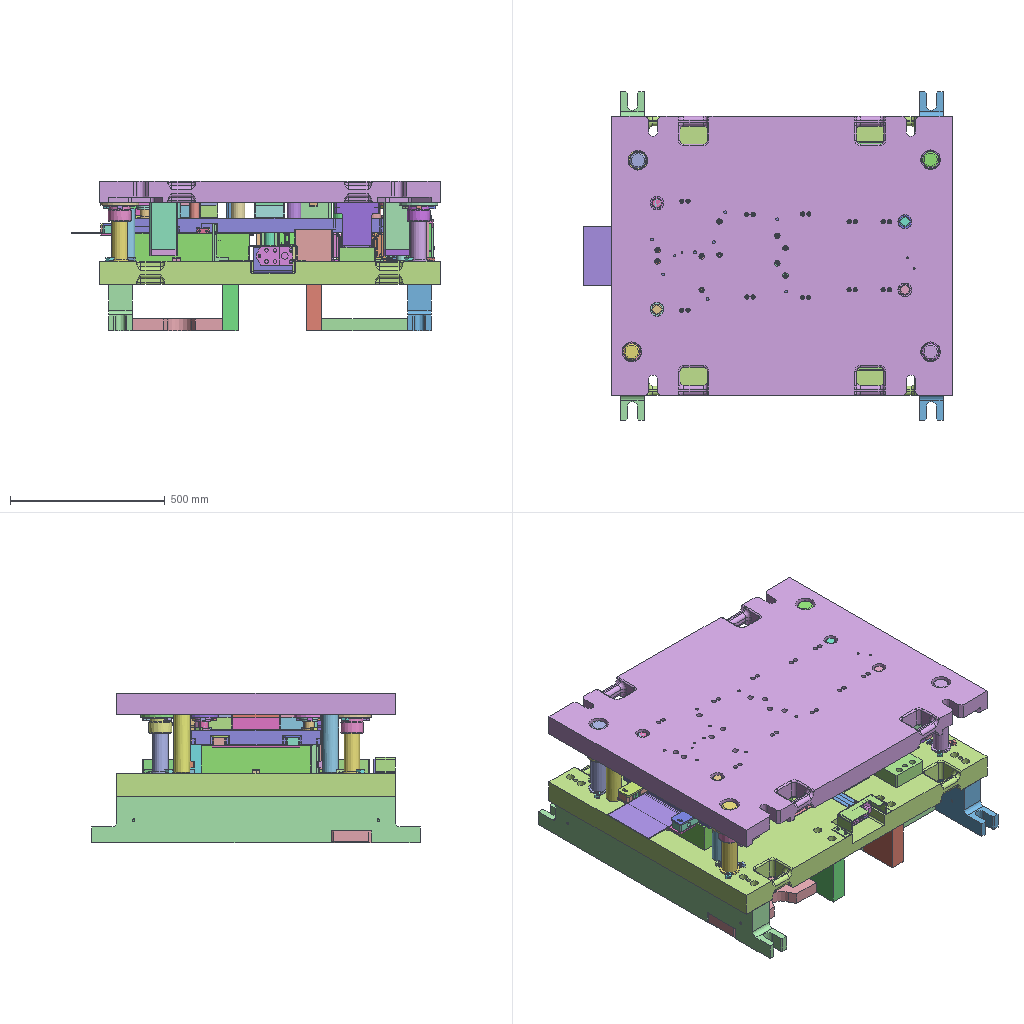Assembly | STEP file | 402 different items | 402 placed | box 1190 x 1060 x 482 mm
Parts list (item | name | quantity | parent item | size | volume):
1 | 1_id1610_x_t | x1 | in 1_x_t | 115 x 159 x 101.122 mm | 1560296 mm3
2 | 1_id1606_x_t | x1 | in 1_x_t | 114.3 x 15 x 55 mm | 89525 mm3
3 | 1_id1602_x_t | x1 | in 1_x_t | 80 x 25 x 25 mm | 40040 mm3
4 | 1_id1598_x_t | x1 | in 1_x_t | 114.3 x 15 x 55 mm | 89525 mm3
5 | 1_id1594_x_t | x1 | in 1_x_t | 15 x 15 x 10 mm | 1899 mm3
6 | 1_id1590_x_t | x1 | in 1_x_t | 61.499 x 105 x 105 mm | 262460 mm3
7 | 1_id1586_x_t | x1 | in 1_x_t | 10 x 35 x 78.24 mm | 2112 mm3
8 | 1_id1582_x_t | x1 | in 1_x_t | 120 x 140.586 x 77.52 mm | 963070 mm3
9 | 1_id1578_x_t | x1 | in 1_x_t | 100 x 20 x 45 mm | 84741 mm3
10 | 1_id1574_x_t | x1 | in 1_x_t | 10 x 10 x 28.4 mm | 1507 mm3
11 | 1_id1570_x_t | x1 | in 1_x_t | 10 x 10 x 28.4 mm | 1507 mm3
12 | 1_id1566_x_t | x1 | in 1_x_t | 10 x 10 x 28.4 mm | 1507 mm3
13 | 1_id1562_x_t | x1 | in 1_x_t | 10 x 10 x 28.4 mm | 1507 mm3
14 | 1_id1558_x_t | x1 | in 1_x_t | 30 x 16 x 16 mm | 6176 mm3
15 | 1_id1554_x_t | x1 | in 1_x_t | 115 x 20 x 66.4 mm | 145757 mm3
16 | 1_id1550_x_t | x1 | in 1_x_t | 95 x 49.497 x 48.669 mm | 78915 mm3
17 | 1_id1546_x_t | x1 | in 1_x_t | 19.05 x 114.3 x 38.1 mm | 57701 mm3
18 | 1_id1542_x_t | x1 | in 1_x_t | 115 x 159 x 101.122 mm | 1560296 mm3
19 | 1_id1538_x_t | x1 | in 1_x_t | 100 x 20 x 45 mm | 84741 mm3
20 | 1_id1534_x_t | x1 | in 1_x_t | 115 x 20 x 66.4 mm | 145757 mm3
21 | 1_id1530_x_t | x1 | in 1_x_t | 50 x 900 x 149.325 mm | 6417398 mm3
22 | 1_id1526_x_t | x1 | in 1_x_t | 63.5 x 25.4 x 25.4 mm | 33278 mm3
23 | 1_id1522_x_t | x1 | in 1_x_t | 63.5 x 25.4 x 25.4 mm | 31340 mm3
24 | 1_id1518_x_t | x1 | in 1_x_t | 303 x 50 x 6 mm | 88049 mm3
25 | 1_id1514_x_t | x1 | in 1_x_t | 31.75 x 19.4 x 24.5 mm | 13370 mm3
26 | 1_id1510_x_t | x1 | in 1_x_t | 243 x 43.296 x 24.5 mm | 189026 mm3
27 | 1_id1506_x_t | x1 | in 1_x_t | 25 x 50 x 20 mm | 19717 mm3
28 | 1_id1502_x_t | x1 | in 1_x_t | 25.4 x 25.4 x 75.5 mm | 37080 mm3
29 | 1_id1498_x_t | x1 | in 1_x_t | 25.4 x 25.4 x 75.5 mm | 37080 mm3
30 | 1_id1494_x_t | x1 | in 1_x_t | 17.227 x 16 x 69.85 mm | 12451 mm3
31 | 1_id1490_x_t | x1 | in 1_x_t | 11 x 11 x 20.4 mm | 1232 mm3
32 | 1_id1486_x_t | x1 | in 1_x_t | 156.936 x 16 x 10 mm | 21479 mm3
33 | 1_id1482_x_t | x1 | in 1_x_t | 90 x 55 x 152 mm | 644176 mm3
34 | 1_id1478_x_t | x1 | in 1_x_t | 90 x 67.5 x 20 mm | 111264 mm3
35 | 1_id1474_x_t | x1 | in 1_x_t | 32 x 32 x 52.035 mm | 37231 mm3
36 | 1_id1470_x_t | x1 | in 1_x_t | 12.7 x 12.7 x 5 mm | 467.469 mm3
37 | 1_id1466_x_t | x1 | in 1_x_t | 10.203 x 31.243 x 10 mm | 1111 mm3
38 | 1_id1462_x_t | x1 | in 1_x_t | 29.76 x 137.606 x 25 mm | 81885 mm3
39 | 1_id1458_x_t | x1 | in 1_x_t | 55 x 60 x 40 mm | 83432 mm3
40 | 1_id1454_x_t | x1 | in 1_x_t | 8 x 7.4 x 20 mm | 828.53 mm3
41 | 1_id1450_x_t | x1 | in 1_x_t | 35.397 x 13.214 x 25 mm | 9704 mm3
42 | 1_id1446_x_t | x1 | in 1_x_t | 25.4 x 38.1 x 121.275 mm | 47668 mm3
43 | 1_id1442_x_t | x1 | in 1_x_t | 10 x 35 x 78.24 mm | 2112 mm3
44 | 1_id1438_x_t | x1 | in 1_x_t | 26.187 x 24.356 x 11 mm | 2271 mm3
45 | 1_id1434_x_t | x1 | in 1_x_t | 26.187 x 24.356 x 11 mm | 2271 mm3
46 | 1_id1430_x_t | x1 | in 1_x_t | 90 x 67.5 x 20 mm | 111264 mm3
47 | 1_id1426_x_t | x1 | in 1_x_t | 90 x 55 x 152 mm | 644176 mm3
48 | 1_id1422_x_t | x1 | in 1_x_t | 90 x 67.5 x 20 mm | 111264 mm3
49 | 1_id1418_x_t | x1 | in 1_x_t | 21 x 16 x 11 mm | 2249 mm3
50 | 1_id1414_x_t | x1 | in 1_x_t | 26.187 x 24.356 x 11 mm | 2271 mm3
51 | 1_id1410_x_t | x1 | in 1_x_t | 39.688 x 39.688 x 146.05 mm | 117725 mm3
52 | 1_id1406_x_t | x1 | in 1_x_t | 26.187 x 24.356 x 11 mm | 2271 mm3
53 | 1_id1402_x_t | x1 | in 1_x_t | 90 x 55 x 152 mm | 644176 mm3
54 | 1_id1398_x_t | x1 | in 1_x_t | 90 x 67.5 x 20 mm | 111264 mm3
55 | 1_id1394_x_t | x1 | in 1_x_t | 90 x 55 x 152 mm | 644176 mm3
56 | 1_id1390_x_t | x1 | in 1_x_t | 26.187 x 24.356 x 11 mm | 2271 mm3
57 | 1_id1386_x_t | x1 | in 1_x_t | 26.187 x 24.356 x 11 mm | 2271 mm3
58 | 1_id1382_x_t | x1 | in 1_x_t | 32 x 32 x 52.035 mm | 37231 mm3
59 | 1_id1378_x_t | x1 | in 1_x_t | 32 x 32 x 52.035 mm | 37231 mm3
60 | 1_id1374_x_t | x1 | in 1_x_t | 39.688 x 39.688 x 146.05 mm | 117725 mm3
61 | 1_id1370_x_t | x1 | in 1_x_t | 26.187 x 24.356 x 11 mm | 2271 mm3
62 | 1_id1366_x_t | x1 | in 1_x_t | 26.187 x 24.356 x 11 mm | 2271 mm3
63 | 1_id1362_x_t | x1 | in 1_x_t | 80 x 25 x 25 mm | 39657 mm3
64 | 1_id1358_x_t | x1 | in 1_x_t | 50.8 x 50.8 x 190.275 mm | 342596 mm3
65 | 1_id1354_x_t | x1 | in 1_x_t | 50.8 x 50.8 x 190.275 mm | 342596 mm3
66 | 1_id1350_x_t | x1 | in 1_x_t | 50.8 x 50.8 x 190.275 mm | 342596 mm3
67 | 1_id1346_x_t | x1 | in 1_x_t | 16 x 21 x 10 mm | 2191 mm3
68 | 1_id1342_x_t | x1 | in 1_x_t | 26.187 x 24.356 x 10 mm | 2191 mm3
69 | 1_id1338_x_t | x1 | in 1_x_t | 50.8 x 50.8 x 190.275 mm | 342596 mm3
70 | 1_id1334_x_t | x1 | in 1_x_t | 20 x 30 x 25 mm | 11989 mm3
71 | 1_id1330_x_t | x1 | in 1_x_t | 209.55 x 63.5 x 50.8 mm | 52722 mm3
72 | 1_id1326_x_t | x1 | in 1_x_t | 75 x 282.347 x 6 mm | 125769 mm3
73 | 1_id1322_x_t | x1 | in 1_x_t | 31.75 x 19.4 x 24.5 mm | 13370 mm3
74 | 1_id1318_x_t | x1 | in 1_x_t | 15 x 15 x 63 mm | 7435 mm3
75 | 1_id1314_x_t | x1 | in 1_x_t | 40.468 x 31 x 10 mm | 8665 mm3
76 | 1_id1310_x_t | x1 | in 1_x_t | 50.8 x 25.4 x 120.024 mm | 43266 mm3
77 | 1_id1306_x_t | x1 | in 1_x_t | 190 x 45 x 2 mm | 16638 mm3
78 | 1_id1302_x_t | x1 | in 1_x_t | 45 x 230 x 2 mm | 20238 mm3
79 | 1_id1298_x_t | x1 | in 1_x_t | 16.123 x 43.759 x 52.166 mm | 26539 mm3
80 | 1_id1294_x_t | x1 | in 1_x_t | 6.655 x 14.782 x 12.7 mm | 658.806 mm3
81 | 1_id1290_x_t | x1 | in 1_x_t | 21.548 x 6.349 x 6.248 mm | 334.04 mm3
82 | 1_id1286_x_t | x1 | in 1_x_t | 10.535 x 11.151 x 36.727 mm | 2077 mm3
83 | 1_id1282_x_t | x1 | in 1_x_t | 41.278 x 12.093 x 11.906 mm | 2345 mm3
84 | 1_id1278_x_t | x1 | in 1_x_t | 21.548 x 6.349 x 6.248 mm | 334.04 mm3
85 | 1_id1274_x_t | x1 | in 1_x_t | 25 x 50 x 20 mm | 19717 mm3
86 | 1_id1270_x_t | x1 | in 1_x_t | 25.206 x 22.218 x 11 mm | 2271 mm3
87 | 1_id1266_x_t | x1 | in 1_x_t | 63.5 x 63.5 x 303.213 mm | 619621 mm3
88 | 1_id1262_x_t | x1 | in 1_x_t | 63.5 x 63.5 x 303.213 mm | 619621 mm3
89 | 1_id1258_x_t | x1 | in 1_x_t | 22.218 x 25.206 x 11 mm | 2271 mm3
90 | 1_id1254_x_t | x1 | in 1_x_t | 23.459 x 19.404 x 11 mm | 2271 mm3
91 | 1_id1250_x_t | x1 | in 1_x_t | 97.332 x 141.374 x 2 mm | 15084 mm3
92 | 1_id1246_x_t | x1 | in 1_x_t | 32 x 32 x 25 mm | 17096 mm3
93 | 1_id1242_x_t | x1 | in 1_x_t | 32 x 32 x 25 mm | 17096 mm3
94 | 1_id1238_x_t | x1 | in 1_x_t | 32 x 32 x 93.24 mm | 66514 mm3
95 | 1_id1234_x_t | x1 | in 1_x_t | 25 x 30 x 25 mm | 14479 mm3
96 | 1_id1230_x_t | x1 | in 1_x_t | 100 x 88.5 x 10 mm | 56263 mm3
97 | 1_id1226_x_t | x1 | in 1_x_t | 95.666 x 100 x 10 mm | 57810 mm3
98 | 1_id1222_x_t | x1 | in 1_x_t | 95.666 x 100 x 10 mm | 57810 mm3
99 | 1_id1218_x_t | x1 | in 1_x_t | 75 x 1060 x 149.325 mm | 10050016 mm3
100 | 1_id1214_x_t | x1 | in 1_x_t | 19.05 x 19.05 x 25.4 mm | 5054 mm3
101 | 1_id1210_x_t | x1 | in 1_x_t | 38 x 115.5 x 38.1 mm | 114761 mm3
102 | 1_id1206_x_t | x1 | in 1_x_t | 11 x 11 x 20.4 mm | 1232 mm3
103 | 1_id1202_x_t | x1 | in 1_x_t | 11 x 11 x 20.4 mm | 1232 mm3
104 | 1_id1198_x_t | x1 | in 1_x_t | 11 x 11 x 20.4 mm | 1232 mm3
105 | 1_id1194_x_t | x1 | in 1_x_t | 11 x 11 x 20.4 mm | 1232 mm3
106 | 1_id1190_x_t | x1 | in 1_x_t | 17.227 x 16 x 69.85 mm | 12451 mm3
107 | 1_id1186_x_t | x1 | in 1_x_t | 164.45 x 32.752 x 20.792 mm | 70018 mm3
108 | 1_id1182_x_t | x1 | in 1_x_t | 163.45 x 32.752 x 20.644 mm | 72190 mm3
109 | 1_id1178_x_t | x1 | in 1_x_t | 19 x 19 x 80 mm | 16778 mm3
110 | 1_id1174_x_t | x1 | in 1_x_t | 17.227 x 16 x 69.85 mm | 12451 mm3
111 | 1_id1170_x_t | x1 | in 1_x_t | 25.7 x 24 x 38.1 mm | 13011 mm3
112 | 1_id1166_x_t | x1 | in 1_x_t | 19 x 19 x 80 mm | 16778 mm3
113 | 1_id1162_x_t | x1 | in 1_x_t | 19 x 19 x 80 mm | 16778 mm3
114 | 1_id1158_x_t | x1 | in 1_x_t | 19 x 19 x 80 mm | 16778 mm3
115 | 1_id1154_x_t | x1 | in 1_x_t | 19 x 19 x 80 mm | 16778 mm3
116 | 1_id1150_x_t | x1 | in 1_x_t | 15.875 x 90.424 x 15.875 mm | 9884 mm3
117 | 1_id1146_x_t | x1 | in 1_x_t | 15.875 x 90.424 x 15.875 mm | 9884 mm3
118 | 1_id1142_x_t | x1 | in 1_x_t | 19 x 62.5 x 19 mm | 15480 mm3
119 | 1_id1138_x_t | x1 | in 1_x_t | 70 x 10 x 37.5 mm | 23507 mm3
120 | 1_id1134_x_t | x1 | in 1_x_t | 31.75 x 19.4 x 24.5 mm | 13370 mm3
121 | 1_id1130_x_t | x1 | in 1_x_t | 32 x 32 x 52.035 mm | 37231 mm3
122 | 1_id1126_x_t | x1 | in 1_x_t | 53.213 x 53.213 x 60.325 mm | 50805 mm3
123 | 1_id1122_x_t | x1 | in 1_x_t | 31.75 x 19.4 x 24.5 mm | 13370 mm3
124 | 1_id1118_x_t | x1 | in 1_x_t | 303 x 43.296 x 24.5 mm | 252825 mm3
125 | 1_id1114_x_t | x1 | in 1_x_t | 26.187 x 24.356 x 11 mm | 2271 mm3
126 | 1_id1110_x_t | x1 | in 1_x_t | 16 x 30 x 16 mm | 6176 mm3
127 | 1_id1106_x_t | x1 | in 1_x_t | 44.5 x 44.5 x 120 mm | 176158 mm3
128 | 1_id1102_x_t | x1 | in 1_x_t | 26.372 x 25.755 x 11 mm | 2271 mm3
129 | 1_id1098_x_t | x1 | in 1_x_t | 26.372 x 25.755 x 11 mm | 2249 mm3
130 | 1_id1094_x_t | x1 | in 1_x_t | 73.936 x 31 x 10 mm | 16212 mm3
131 | 1_id1090_x_t | x1 | in 1_x_t | 20.89 x 24.426 x 11 mm | 2271 mm3
132 | 1_id1086_x_t | x1 | in 1_x_t | 24.356 x 26.187 x 11 mm | 2249 mm3
133 | 1_id1082_x_t | x1 | in 1_x_t | 39.688 x 39.688 x 146.05 mm | 117725 mm3
134 | 1_id1078_x_t | x1 | in 1_x_t | 26.187 x 24.356 x 11 mm | 2271 mm3
135 | 1_id1074_x_t | x1 | in 1_x_t | 31.75 x 19.4 x 24.5 mm | 13473 mm3
136 | 1_id1070_x_t | x1 | in 1_x_t | 25.755 x 26.372 x 11 mm | 2271 mm3
137 | 1_id1066_x_t | x1 | in 1_x_t | 26.187 x 24.356 x 11 mm | 2271 mm3
138 | 1_id1062_x_t | x1 | in 1_x_t | 53.213 x 53.213 x 41.275 mm | 36326 mm3
139 | 1_id1058_x_t | x1 | in 1_x_t | 13.4 x 15.898 x 28.911 mm | 4184 mm3
140 | 1_id1054_x_t | x1 | in 1_x_t | 25 x 30 x 25 mm | 14479 mm3
141 | 1_id1050_x_t | x1 | in 1_x_t | 26.187 x 24.356 x 11 mm | 2271 mm3
142 | 1_id1046_x_t | x1 | in 1_x_t | 80 x 25 x 25 mm | 39657 mm3
143 | 1_id1042_x_t | x1 | in 1_x_t | 77.8 x 77.8 x 92.075 mm | 159468 mm3
144 | 1_id1038_x_t | x1 | in 1_x_t | 24.356 x 26.187 x 11 mm | 2249 mm3
145 | 1_id1034_x_t | x1 | in 1_x_t | 21 x 16 x 11 mm | 2249 mm3
146 | 1_id1030_x_t | x1 | in 1_x_t | 80 x 25 x 25 mm | 39657 mm3
147 | 1_id1026_x_t | x1 | in 1_x_t | 80 x 15 x 43 mm | 46403 mm3
148 | 1_id1022_x_t | x1 | in 1_x_t | 26.372 x 25.755 x 11 mm | 2249 mm3
149 | 1_id1018_x_t | x1 | in 1_x_t | 21 x 16 x 11 mm | 2249 mm3
150 | 1_id1014_x_t | x1 | in 1_x_t | 24.356 x 26.187 x 11 mm | 2249 mm3
151 | 1_id1010_x_t | x1 | in 1_x_t | 25.4 x 25.4 x 75.5 mm | 37080 mm3
152 | 1_id1006_x_t | x1 | in 1_x_t | 10 x 10 x 28.4 mm | 1507 mm3
153 | 1_id1002_x_t | x1 | in 1_x_t | 36.508 x 90.344 x 25 mm | 24887 mm3
154 | 1_id998_x_t | x1 | in 1_x_t | 82.5 x 86.2 x 38.01 mm | 245705 mm3
155 | 1_id994_x_t | x1 | in 1_x_t | 70 x 43.296 x 26 mm | 59877 mm3
156 | 1_id990_x_t | x1 | in 1_x_t | 21 x 16 x 11 mm | 2249 mm3
157 | 1_id986_x_t | x1 | in 1_x_t | 31.75 x 19.4 x 24.5 mm | 13370 mm3
158 | 1_id982_x_t | x1 | in 1_x_t | 15.875 x 15.875 x 5.08 mm | 809.996 mm3
159 | 1_id978_x_t | x1 | in 1_x_t | 243 x 50 x 6 mm | 70049 mm3
160 | 1_id974_x_t | x1 | in 1_x_t | 19.404 x 23.459 x 11 mm | 2271 mm3
161 | 1_id970_x_t | x1 | in 1_x_t | 25.4 x 25.4 x 75.5 mm | 37080 mm3
162 | 1_id966_x_t | x1 | in 1_x_t | 26.372 x 25.755 x 11 mm | 2271 mm3
163 | 1_id962_x_t | x1 | in 1_x_t | 50 x 25 x 20 mm | 19717 mm3
164 | 1_id958_x_t | x1 | in 1_x_t | 19 x 19 x 80 mm | 16778 mm3
165 | 1_id954_x_t | x1 | in 1_x_t | 10 x 10 x 28.4 mm | 1507 mm3
166 | 1_id950_x_t | x1 | in 1_x_t | 417 x 130 x 38.1 mm | 1861233 mm3
167 | 1_id946_x_t | x1 | in 1_x_t | 25.206 x 22.218 x 11 mm | 2271 mm3
168 | 1_id942_x_t | x1 | in 1_x_t | 19 x 19 x 80 mm | 16778 mm3
169 | 1_id938_x_t | x1 | in 1_x_t | 15.875 x 15.875 x 5.08 mm | 809.996 mm3
170 | 1_id934_x_t | x1 | in 1_x_t | 19 x 19 x 80 mm | 16778 mm3
171 | 1_id930_x_t | x1 | in 1_x_t | 26.372 x 25.755 x 11 mm | 2249 mm3
172 | 1_id926_x_t | x1 | in 1_x_t | 19 x 19 x 80 mm | 16778 mm3
173 | 1_id922_x_t | x1 | in 1_x_t | 15.876 x 15.876 x 5 mm | 818.728 mm3
174 | 1_id918_x_t | x1 | in 1_x_t | 7.4 x 8 x 20 mm | 828.53 mm3
175 | 1_id914_x_t | x1 | in 1_x_t | 15.875 x 15.875 x 5.08 mm | 809.996 mm3
176 | 1_id910_x_t | x1 | in 1_x_t | 10 x 10 x 28.4 mm | 1507 mm3
177 | 1_id906_x_t | x1 | in 1_x_t | 17 x 15 x 10 mm | 2199 mm3
178 | 1_id902_x_t | x1 | in 1_x_t | 12.423 x 12.423 x 53.975 mm | 6543 mm3
179 | 1_id898_x_t | x1 | in 1_x_t | 25.206 x 22.218 x 11 mm | 2271 mm3
180 | 1_id894_x_t | x1 | in 1_x_t | 19 x 19 x 80 mm | 16778 mm3
181 | 1_id890_x_t | x1 | in 1_x_t | 80 x 25 x 25 mm | 40040 mm3
182 | 1_id886_x_t | x1 | in 1_x_t | 15 x 15 x 10 mm | 1899 mm3
183 | 1_id882_x_t | x1 | in 1_x_t | 26.372 x 25.755 x 11 mm | 2271 mm3
184 | 1_id878_x_t | x1 | in 1_x_t | 19 x 19 x 80 mm | 16778 mm3
185 | 1_id874_x_t | x1 | in 1_x_t | 80 x 15 x 43 mm | 46403 mm3
186 | 1_id870_x_t | x1 | in 1_x_t | 4.715 x 9.009 x 51.008 mm | 844.246 mm3
187 | 1_id866_x_t | x1 | in 1_x_t | 70 x 10 x 37.5 mm | 23507 mm3
188 | 1_id862_x_t | x1 | in 1_x_t | 19.404 x 23.459 x 11 mm | 2271 mm3
189 | 1_id858_x_t | x1 | in 1_x_t | 30 x 23 x 45 mm | 21294 mm3
190 | 1_id854_x_t | x1 | in 1_x_t | 12.7 x 12.7 x 5 mm | 467.469 mm3
191 | 1_id850_x_t | x1 | in 1_x_t | 26.187 x 24.356 x 11 mm | 2271 mm3
192 | 1_id846_x_t | x1 | in 1_x_t | 17 x 15 x 10 mm | 2199 mm3
193 | 1_id842_x_t | x1 | in 1_x_t | 30 x 23 x 45 mm | 21294 mm3
194 | 1_id838_x_t | x1 | in 1_x_t | 120 x 140.586 x 77.52 mm | 963070 mm3
195 | 1_id834_x_t | x1 | in 1_x_t | 114.4 x 115 x 102.9 mm | 813776 mm3
196 | 1_id830_x_t | x1 | in 1_x_t | 26.187 x 24.356 x 11 mm | 2271 mm3
197 | 1_id826_x_t | x1 | in 1_x_t | 17.227 x 16 x 69.85 mm | 12451 mm3
198 | 1_id822_x_t | x1 | in 1_x_t | 19 x 58.09 x 19 mm | 14020 mm3
199 | 1_id818_x_t | x1 | in 1_x_t | 80 x 60 x 119 mm | 412634 mm3
200 | 1_id814_x_t | x1 | in 1_x_t | 19 x 58.09 x 19 mm | 14020 mm3
201 | 1_id810_x_t | x1 | in 1_x_t | 26.07 x 24 x 38.1 mm | 13100 mm3
202 | 1_id806_x_t | x1 | in 1_x_t | 97.332 x 141.374 x 2 mm | 15921 mm3
203 | 1_id802_x_t | x1 | in 1_x_t | 100 x 85.5 x 10 mm | 54246 mm3
204 | 1_id798_x_t | x1 | in 1_x_t | 11 x 11 x 20.4 mm | 1232 mm3
205 | 1_id794_x_t | x1 | in 1_x_t | 15.875 x 15.875 x 5.08 mm | 809.996 mm3
206 | 1_id790_x_t | x1 | in 1_x_t | 5.952 x 155.177 x 73.747 mm | 311.788 mm3
207 | 1_id786_x_t | x1 | in 1_x_t | 26.767 x 58.14 x 102.478 mm | 28325 mm3
208 | 1_id782_x_t | x1 | in 1_x_t | 11 x 11 x 20.4 mm | 1232 mm3
209 | 1_id778_x_t | x1 | in 1_x_t | 80 x 25 x 25 mm | 40040 mm3
210 | 1_id774_x_t | x1 | in 1_x_t | 26.372 x 25.755 x 11 mm | 2249 mm3
211 | 1_id770_x_t | x1 | in 1_x_t | 53.213 x 53.213 x 60.325 mm | 50805 mm3
212 | 1_id766_x_t | x1 | in 1_x_t | 15.875 x 15.875 x 5.08 mm | 809.996 mm3
213 | 1_id762_x_t | x1 | in 1_x_t | 50 x 900 x 149.325 mm | 6424966 mm3
214 | 1_id758_x_t | x1 | in 1_x_t | 63.5 x 63.5 x 303.213 mm | 619621 mm3
215 | 1_id754_x_t | x1 | in 1_x_t | 25.4 x 25.4 x 75.5 mm | 37080 mm3
216 | 1_id750_x_t | x1 | in 1_x_t | 15.875 x 15.875 x 5.08 mm | 809.996 mm3
217 | 1_id746_x_t | x1 | in 1_x_t | 10 x 10 x 28.4 mm | 1507 mm3
218 | 1_id742_x_t | x1 | in 1_x_t | 39.688 x 39.688 x 146.05 mm | 117725 mm3
219 | 1_id738_x_t | x1 | in 1_x_t | 24.356 x 26.187 x 11 mm | 2249 mm3
220 | 1_id734_x_t | x1 | in 1_x_t | 75 x 1060 x 149.325 mm | 10048750 mm3
221 | 1_id730_x_t | x1 | in 1_x_t | 32 x 32 x 93.24 mm | 66514 mm3
222 | 1_id726_x_t | x1 | in 1_x_t | 15 x 102.012 x 118 mm | 27733 mm3
223 | 1_id722_x_t | x1 | in 1_x_t | 25.4 x 25.4 x 75.5 mm | 37080 mm3
224 | 1_id718_x_t | x1 | in 1_x_t | 118 x 27.94 x 59.944 mm | 104639 mm3
225 | 1_id714_x_t | x1 | in 1_x_t | 32 x 32 x 93.24 mm | 66514 mm3
226 | 1_id710_x_t | x1 | in 1_x_t | 80 x 25 x 25 mm | 40040 mm3
227 | 1_id706_x_t | x1 | in 1_x_t | 127 x 29.369 x 82.55 mm | 82680 mm3
228 | 1_id702_x_t | x1 | in 1_x_t | 63.5 x 63.5 x 303.213 mm | 619621 mm3
229 | 1_id698_x_t | x1 | in 1_x_t | 39.688 x 39.688 x 146.05 mm | 117725 mm3
230 | 1_id694_x_t | x1 | in 1_x_t | 32 x 32 x 93.24 mm | 66514 mm3
231 | 1_id690_x_t | x1 | in 1_x_t | 32 x 92 x 31.644 mm | 71708 mm3
232 | 1_id686_x_t | x1 | in 1_x_t | 80 x 25 x 25 mm | 39657 mm3
233 | 1_id682_x_t | x1 | in 1_x_t | 56 x 128.26 x 99.32 mm | 209835 mm3
234 | 1_id678_x_t | x1 | in 1_x_t | 95 x 49.497 x 48.669 mm | 78915 mm3
235 | 1_id674_x_t | x1 | in 1_x_t | 10.203 x 31.243 x 10 mm | 1111 mm3
236 | 1_id670_x_t | x1 | in 1_x_t | 44 x 25 x 107.009 mm | 59060 mm3
237 | 1_id666_x_t | x1 | in 1_x_t | 11 x 11 x 20.4 mm | 1232 mm3
238 | 1_id662_x_t | x1 | in 1_x_t | 53.213 x 53.213 x 60.325 mm | 50805 mm3
239 | 1_id658_x_t | x1 | in 1_x_t | 69.088 x 69.85 x 41.275 mm | 100264 mm3
240 | 1_id654_x_t | x1 | in 1_x_t | 31.75 x 31.75 x 101.6 mm | 61988 mm3
241 | 1_id650_x_t | x1 | in 1_x_t | 403 x 130 x 38.1 mm | 1939605 mm3
242 | 1_id646_x_t | x1 | in 1_x_t | 49 x 79 x 5 mm | 17399 mm3
243 | 1_id642_x_t | x1 | in 1_x_t | 35 x 200 x 2 mm | 12091 mm3
244 | 1_id638_x_t | x1 | in 1_x_t | 149 x 35 x 2 mm | 8095 mm3
245 | 1_id634_x_t | x1 | in 1_x_t | 149 x 35 x 2 mm | 8095 mm3
246 | 1_id630_x_t | x1 | in 1_x_t | 44 x 25 x 107.009 mm | 59060 mm3
247 | 1_id626_x_t | x1 | in 1_x_t | 35 x 137 x 38.1 mm | 136243 mm3
248 | 1_id622_x_t | x1 | in 1_x_t | 168 x 137 x 20 mm | 442179 mm3
249 | 1_id618_x_t | x1 | in 1_x_t | 19 x 58.09 x 19 mm | 14020 mm3
250 | 1_id614_x_t | x1 | in 1_x_t | 19 x 58.09 x 19 mm | 14020 mm3
251 | 1_id610_x_t | x1 | in 1_x_t | 71 x 8 x 72 mm | 30523 mm3
252 | 1_id606_x_t | x1 | in 1_x_t | 19 x 58.09 x 19 mm | 14020 mm3
253 | 1_id602_x_t | x1 | in 1_x_t | 19 x 62.5 x 19 mm | 15480 mm3
254 | 1_id598_x_t | x1 | in 1_x_t | 35 x 137 x 38.1 mm | 136243 mm3
255 | 1_id594_x_t | x1 | in 1_x_t | 71 x 35 x 72 mm | 118326 mm3
256 | 1_id590_x_t | x1 | in 1_x_t | 15.875 x 90.424 x 15.875 mm | 9884 mm3
257 | 1_id586_x_t | x1 | in 1_x_t | 15.875 x 90.424 x 15.875 mm | 9884 mm3
258 | 1_id582_x_t | x1 | in 1_x_t | 35 x 137 x 38.1 mm | 136243 mm3
259 | 1_id578_x_t | x1 | in 1_x_t | 168 x 137 x 20 mm | 442179 mm3
260 | 1_id574_x_t | x1 | in 1_x_t | 19 x 58.09 x 19 mm | 14020 mm3
261 | 1_id570_x_t | x1 | in 1_x_t | 71 x 8 x 72 mm | 30523 mm3
262 | 1_id566_x_t | x1 | in 1_x_t | 35 x 137 x 38.1 mm | 136243 mm3
263 | 1_id562_x_t | x1 | in 1_x_t | 71 x 35 x 72 mm | 118326 mm3
264 | 1_id558_x_t | x1 | in 1_x_t | 19.05 x 114.3 x 38.1 mm | 57701 mm3
265 | 1_id554_x_t | x1 | in 1_x_t | 114.4 x 115 x 102.9 mm | 813776 mm3
266 | 1_id550_x_t | x1 | in 1_x_t | 19.05 x 114.3 x 38.1 mm | 57701 mm3
267 | 1_id546_x_t | x1 | in 1_x_t | 19.05 x 114.3 x 38.1 mm | 57701 mm3
268 | 1_id542_x_t | x1 | in 1_x_t | 11 x 11 x 20.4 mm | 1232 mm3
269 | 1_id538_x_t | x1 | in 1_x_t | 162.45 x 32.752 x 10 mm | 49655 mm3
270 | 1_id534_x_t | x1 | in 1_x_t | 163.45 x 32.752 x 10 mm | 50026 mm3
271 | 1_id530_x_t | x1 | in 1_x_t | 11 x 11 x 20.4 mm | 1232 mm3
272 | 1_id526_x_t | x1 | in 1_x_t | 11 x 11 x 20.4 mm | 1232 mm3
273 | 1_id522_x_t | x1 | in 1_x_t | 11 x 11 x 20.4 mm | 1232 mm3
274 | 1_id518_x_t | x1 | in 1_x_t | 11 x 11 x 20.4 mm | 1232 mm3
275 | 1_id514_x_t | x1 | in 1_x_t | 11 x 11 x 20.4 mm | 1232 mm3
276 | 1_id510_x_t | x1 | in 1_x_t | 11 x 11 x 20.4 mm | 1232 mm3
277 | 1_id506_x_t | x1 | in 1_x_t | 11 x 11 x 20.4 mm | 1232 mm3
278 | 1_id502_x_t | x1 | in 1_x_t | 11 x 11 x 20.4 mm | 1232 mm3
279 | 1_id498_x_t | x1 | in 1_x_t | 11 x 11 x 20.4 mm | 1232 mm3
280 | 1_id494_x_t | x1 | in 1_x_t | 11 x 11 x 20.4 mm | 1232 mm3
281 | 1_id490_x_t | x1 | in 1_x_t | 11 x 11 x 20.4 mm | 1232 mm3
282 | 1_id486_x_t | x1 | in 1_x_t | 50.8 x 50.038 x 41.275 mm | 56529 mm3
283 | 1_id482_x_t | x1 | in 1_x_t | 12.7 x 12.7 x 103.124 mm | 10701 mm3
284 | 1_id478_x_t | x1 | in 1_x_t | 125 x 105 x 10 mm | 77042 mm3
285 | 1_id474_x_t | x1 | in 1_x_t | 44.5 x 44.5 x 120 mm | 176158 mm3
286 | 1_id470_x_t | x1 | in 1_x_t | 44.5 x 44.5 x 120 mm | 176158 mm3
287 | 1_id466_x_t | x1 | in 1_x_t | 44.5 x 44.5 x 120 mm | 176158 mm3
288 | 1_id462_x_t | x1 | in 1_x_t | 44.5 x 44.5 x 120 mm | 176158 mm3
289 | 1_id458_x_t | x1 | in 1_x_t | 44.5 x 44.5 x 120 mm | 176158 mm3
290 | 1_id454_x_t | x1 | in 1_x_t | 44.5 x 44.5 x 120 mm | 176158 mm3
291 | 1_id450_x_t | x1 | in 1_x_t | 44.5 x 44.5 x 120 mm | 176158 mm3
292 | 1_id446_x_t | x1 | in 1_x_t | 44.5 x 44.5 x 120 mm | 176158 mm3
293 | 1_id442_x_t | x1 | in 1_x_t | 44.5 x 44.5 x 120 mm | 176158 mm3
294 | 1_id438_x_t | x1 | in 1_x_t | 26.187 x 24.356 x 10 mm | 2191 mm3
295 | 1_id434_x_t | x1 | in 1_x_t | 26.187 x 24.356 x 10 mm | 2191 mm3
296 | 1_id430_x_t | x1 | in 1_x_t | 125 x 105 x 10 mm | 77042 mm3
297 | 1_id426_x_t | x1 | in 1_x_t | 26.187 x 24.356 x 10 mm | 2191 mm3
298 | 1_id422_x_t | x1 | in 1_x_t | 16 x 21 x 10 mm | 2191 mm3
299 | 1_id418_x_t | x1 | in 1_x_t | 77.8 x 77.8 x 92.075 mm | 159468 mm3
300 | 1_id414_x_t | x1 | in 1_x_t | 77.8 x 77.8 x 92.075 mm | 159468 mm3
301 | 1_id410_x_t | x1 | in 1_x_t | 125 x 105 x 10 mm | 77042 mm3
302 | 1_id406_x_t | x1 | in 1_x_t | 16 x 21 x 10 mm | 2191 mm3
303 | 1_id402_x_t | x1 | in 1_x_t | 26.187 x 24.356 x 10 mm | 2191 mm3
304 | 1_id398_x_t | x1 | in 1_x_t | 26.187 x 24.356 x 10 mm | 2191 mm3
305 | 1_id394_x_t | x1 | in 1_x_t | 77.8 x 77.8 x 92.075 mm | 159468 mm3
306 | 1_id390_x_t | x1 | in 1_x_t | 26.187 x 24.356 x 10 mm | 2191 mm3
307 | 1_id386_x_t | x1 | in 1_x_t | 125 x 105 x 10 mm | 77042 mm3
308 | 1_id382_x_t | x1 | in 1_x_t | 16 x 21 x 10 mm | 2191 mm3
309 | 1_id378_x_t | x1 | in 1_x_t | 26.187 x 24.356 x 10 mm | 2191 mm3
310 | 1_id374_x_t | x1 | in 1_x_t | 68.793 x 69.35 x 5 mm | 16032 mm3
311 | 1_id370_x_t | x1 | in 1_x_t | 9.15 x 21.764 x 3.075 mm | 435.444 mm3
312 | 1_id366_x_t | x1 | in 1_x_t | 48.382 x 188.49 x 8.554 mm | 28332 mm3
313 | 1_id362_x_t | x1 | in 1_x_t | 8.17 x 3.075 x 8.17 mm | 161.205 mm3
314 | PARTBODY_id358_x_t | x1 | in 1_x_t | 48 x 47.1 x 81.415 mm | 28561 mm3
315 | PARTBODY_id354_x_t | x1 | in 1_x_t | 48 x 47.1 x 81.415 mm | 28561 mm3
316 | 1_id350_x_t | x1 | in 1_x_t | 8.17 x 3.075 x 8.17 mm | 161.205 mm3
317 | 1_id346_x_t | x1 | in 1_x_t | 48.382 x 188.49 x 8.554 mm | 28333 mm3
318 | 1_id342_x_t | x1 | in 1_x_t | 8.17 x 3.075 x 8.17 mm | 161.205 mm3
319 | 1_id338_x_t | x1 | in 1_x_t | 9.576 x 9.576 x 3.075 mm | 221.455 mm3
320 | PARTBODY_id334_x_t | x1 | in 1_x_t | 48 x 47.1 x 81.415 mm | 28561 mm3
321 | PARTBODY_id330_x_t | x1 | in 1_x_t | 48 x 46.9 x 81.415 mm | 29174 mm3
322 | 1_id326_x_t | x1 | in 1_x_t | 9.576 x 9.576 x 3.075 mm | 221.455 mm3
323 | 1_id322_x_t | x1 | in 1_x_t | 8.17 x 3.075 x 8.17 mm | 161.205 mm3
324 | 1_id318_x_t | x1 | in 1_x_t | 8.17 x 3.075 x 8.17 mm | 161.205 mm3
325 | PARTBODY_id314_x_t | x1 | in 1_x_t | 48 x 48.7 x 81.415 mm | 29466 mm3
326 | PARTBODY_id310_x_t | x1 | in 1_x_t | 48 x 47.1 x 81.415 mm | 29206 mm3
327 | 1_id306_x_t | x1 | in 1_x_t | 8.17 x 3.075 x 8.17 mm | 161.205 mm3
328 | 1_id302_x_t | x1 | in 1_x_t | 8.17 x 3.075 x 8.17 mm | 161.205 mm3
329 | 1_id298_x_t | x1 | in 1_x_t | 499.877 x 188.495 x 8.554 mm | 279674 mm3
330 | PARTBODY_id294_x_t | x1 | in 1_x_t | 48 x 47.1 x 81.415 mm | 29206 mm3
331 | 1_id290_x_t | x1 | in 1_x_t | 4.043 x 0.7546 x 0.00007192 mm | 0.000006524 mm3
332 | 1_id286_x_t | x1 | in 1_x_t | 8.95 x 3 x 8.95 mm | 188.737 mm3
333 | 1_id282_x_t | x1 | in 1_x_t | 143.3 x 84 x 105 mm | 430781 mm3
334 | 1_id278_x_t | x1 | in 1_x_t | 13 x 14 x 43 mm | 5330 mm3
335 | 1_id274_x_t | x1 | in 1_x_t | 13 x 14 x 43 mm | 5330 mm3
336 | 1_id270_x_t | x1 | in 1_x_t | 20 x 20 x 20 mm | 5374 mm3
337 | 1_id266_x_t | x1 | in 1_x_t | 70.8 x 244.8 x 3 mm | 48416 mm3
338 | 1_id262_x_t | x1 | in 1_x_t | 11 x 11 x 48.205 mm | 3006 mm3
339 | 1_id258_x_t | x1 | in 1_x_t | 11 x 11 x 4 mm | 380.137 mm3
340 | 1_id254_x_t | x1 | in 1_x_t | 11 x 11 x 48.205 mm | 3006 mm3
341 | 1_id250_x_t | x1 | in 1_x_t | 11 x 11 x 48.205 mm | 3006 mm3
342 | 1_id246_x_t | x1 | in 1_x_t | 11 x 11 x 48.205 mm | 3006 mm3
343 | 1_id242_x_t | x1 | in 1_x_t | 11 x 11 x 48.205 mm | 3006 mm3
344 | 1_id238_x_t | x1 | in 1_x_t | 11 x 11 x 48.205 mm | 3006 mm3
345 | 1_id234_x_t | x1 | in 1_x_t | 11 x 11 x 48.205 mm | 3006 mm3
346 | 1_id230_x_t | x1 | in 1_x_t | 11 x 11 x 48.205 mm | 3006 mm3
347 | 1_id226_x_t | x1 | in 1_x_t | 11 x 11 x 48.205 mm | 3006 mm3
348 | 1_id222_x_t | x1 | in 1_x_t | 11 x 11 x 48.205 mm | 3006 mm3
349 | 1_id218_x_t | x1 | in 1_x_t | 11 x 11 x 48.205 mm | 3006 mm3
350 | 1_id214_x_t | x1 | in 1_x_t | 11 x 11 x 48.205 mm | 3006 mm3
351 | 1_id210_x_t | x1 | in 1_x_t | 48 x 173.045 x 42.999 mm | 28963 mm3
352 | 1_id206_x_t | x1 | in 1_x_t | 68 x 186 x 10 mm | 120598 mm3
353 | 1_id202_x_t | x1 | in 1_x_t | 68 x 186 x 38.1 mm | 377160 mm3
354 | 1_id198_x_t | x1 | in 1_x_t | 51.017 x 50.028 x 5 mm | 8124 mm3
355 | 1_id194_x_t | x1 | in 1_x_t | 1100 x 900 x 68 mm | 61756631 mm3
356 | 1_id190_x_t | x1 | in 1_x_t | 98 x 265 x 10 mm | 250017 mm3
357 | 1_id186_x_t | x1 | in 1_x_t | 68 x 155 x 10 mm | 99518 mm3
358 | 1_id182_x_t | x1 | in 1_x_t | 68 x 185 x 10 mm | 112684 mm3
359 | 1_id178_x_t | x1 | in 1_x_t | 68 x 185 x 38.1 mm | 347953 mm3
360 | 1_id174_x_t | x1 | in 1_x_t | 68 x 155 x 38.1 mm | 290380 mm3
361 | 1_id170_x_t | x1 | in 1_x_t | 98 x 265 x 38.1 mm | 540767 mm3
362 | 1_id166_x_t | x1 | in 1_x_t | 145 x 95 x 182.773 mm | 1439851 mm3
363 | 1_id162_x_t | x1 | in 1_x_t | 145 x 95 x 182.773 mm | 1440904 mm3
364 | 1_id158_x_t | x1 | in 1_x_t | 114.3 x 103.32 x 163.553 mm | 1068364 mm3
365 | 1_id154_x_t | x1 | in 1_x_t | 114.3 x 103.32 x 163.553 mm | 1067173 mm3
366 | 1_id150_x_t | x1 | in 1_x_t | 51 x 202 x 97.035 mm | 913093 mm3
367 | 1_id146_x_t | x1 | in 1_x_t | 35 x 131.5 x 97.111 mm | 189227 mm3
368 | 1_id142_x_t | x1 | in 1_x_t | 35 x 130.5 x 97.111 mm | 188320 mm3
369 | 1_id138_x_t | x1 | in 1_x_t | 36 x 66 x 86.679 mm | 191132 mm3
370 | 1_id134_x_t | x1 | in 1_x_t | 35.8 x 65.8 x 6 mm | 12762 mm3
371 | 1_id130_x_t | x1 | in 1_x_t | 925 x 416 x 45.006 mm | 11838970 mm3
372 | 1_id126_x_t | x1 | in 1_x_t | 400 x 355 x 90 mm | 10202987 mm3
373 | 1_id122_x_t | x1 | in 1_x_t | 35 x 115.5 x 38.1 mm | 107010 mm3
374 | 1_id118_x_t | x1 | in 1_x_t | 96 x 38 x 70.5 mm | 174436 mm3
375 | 1_id114_x_t | x1 | in 1_x_t | 71 x 245 x 22.4 mm | 320775 mm3
376 | 1_id110_x_t | x1 | in 1_x_t | 35 x 115.5 x 38.1 mm | 106763 mm3
377 | 1_id106_x_t | x1 | in 1_x_t | 38 x 115.5 x 38.1 mm | 113928 mm3
378 | 1_id102_x_t | x1 | in 1_x_t | 50 x 80 x 38.1 mm | 121881 mm3
379 | 1_id98_x_t | x1 | in 1_x_t | 96 x 38 x 70.5 mm | 174436 mm3
380 | 1_id94_x_t | x1 | in 1_x_t | 1100 x 900 x 75 mm | 64161476 mm3
381 | 1_id90_x_t | x1 | in 1_x_t | 48 x 173.045 x 42.934 mm | 28634 mm3
382 | 1_id86_x_t | x1 | in 1_x_t | 48 x 173.045 x 42.999 mm | 28624 mm3
383 | 1_id82_x_t | x1 | in 1_x_t | 80 x 230 x 101 mm | 1363447 mm3
384 | 1_id78_x_t | x1 | in 1_x_t | 80 x 230 x 4 mm | 72058 mm3
385 | 1_id74_x_t | x1 | in 1_x_t | 56 x 195 x 126 mm | 1101348 mm3
386 | 1_id70_x_t | x1 | in 1_x_t | 56 x 195 x 4.5 mm | 48168 mm3
387 | 1_id66_x_t | x1 | in 1_x_t | 48 x 173.045 x 42.999 mm | 28624 mm3
388 | 1_id62_x_t | x1 | in 1_x_t | 72 x 85 x 105 mm | 283891 mm3
389 | 1_id58_x_t | x1 | in 1_x_t | 66 x 85 x 105 mm | 245163 mm3
390 | 1_id54_x_t | x1 | in 1_x_t | 57.15 x 38 x 85.5 mm | 141794 mm3
391 | 1_id50_x_t | x1 | in 1_x_t | 57.15 x 38 x 85.5 mm | 143205 mm3
392 | 1_id46_x_t | x1 | in 1_x_t | 57.15 x 38 x 85.5 mm | 141792 mm3
393 | 1_id42_x_t | x1 | in 1_x_t | 57.15 x 38 x 85.5 mm | 143246 mm3
394 | 1_id38_x_t | x1 | in 1_x_t | 9.15 x 21.764 x 3.075 mm | 435.444 mm3
395 | 1_id34_x_t | x1 | in 1_x_t | 9.15 x 21.764 x 3.075 mm | 435.444 mm3
396 | 1_id30_x_t | x1 | in 1_x_t | 9.15 x 21.764 x 3.075 mm | 435.444 mm3
397 | 1_id26_x_t | x1 | in 1_x_t | 9.15 x 21.764 x 3.075 mm | 435.444 mm3
398 | 1_id22_x_t | x1 | in 1_x_t | 9.15 x 21.764 x 3.075 mm | 435.444 mm3
399 | 1_id18_x_t | x1 | in 1_x_t | 9.15 x 21.764 x 3.075 mm | 435.444 mm3
400 | 1_id14_x_t | x1 | in 1_x_t | 9.15 x 21.764 x 3.075 mm | 435.444 mm3
401 | 1_id10_x_t | x1 | in 1_x_t | 9.15 x 21.764 x 3.075 mm | 435.444 mm3
402 | 1_id6_x_t | x1 | in 1_x_t | 9.15 x 21.764 x 3.075 mm | 435.444 mm3
Placements (level | parent | child | x y z in mm | rotation matrix by rows), first 180 of 402 lines:
1 | 1_x_t | 1_id1610_x_t | 0.0 0.0 0.0 | 1 0 0 0 1 0 0 0 1
1 | 1_x_t | 1_id1606_x_t | 0.0 0.0 0.0 | 1 0 0 0 1 0 0 0 1
1 | 1_x_t | 1_id1602_x_t | 0.0 0.0 0.0 | 1 0 0 0 1 0 0 0 1
1 | 1_x_t | 1_id1598_x_t | 0.0 0.0 0.0 | 1 0 0 0 1 0 0 0 1
1 | 1_x_t | 1_id1594_x_t | 0.0 0.0 0.0 | 1 0 0 0 1 0 0 0 1
1 | 1_x_t | 1_id1590_x_t | 0.0 0.0 0.0 | 1 0 0 0 1 0 0 0 1
1 | 1_x_t | 1_id1586_x_t | 0.0 0.0 0.0 | 1 0 0 0 1 0 0 0 1
1 | 1_x_t | 1_id1582_x_t | 0.0 0.0 0.0 | 1 0 0 0 1 0 0 0 1
1 | 1_x_t | 1_id1578_x_t | 0.0 0.0 0.0 | 1 0 0 0 1 0 0 0 1
1 | 1_x_t | 1_id1574_x_t | 0.0 0.0 0.0 | 1 0 0 0 1 0 0 0 1
1 | 1_x_t | 1_id1570_x_t | 0.0 0.0 0.0 | 1 0 0 0 1 0 0 0 1
1 | 1_x_t | 1_id1566_x_t | 0.0 0.0 0.0 | 1 0 0 0 1 0 0 0 1
1 | 1_x_t | 1_id1562_x_t | 0.0 0.0 0.0 | 1 0 0 0 1 0 0 0 1
1 | 1_x_t | 1_id1558_x_t | 0.0 0.0 0.0 | 1 0 0 0 1 0 0 0 1
1 | 1_x_t | 1_id1554_x_t | 0.0 0.0 0.0 | 1 0 0 0 1 0 0 0 1
1 | 1_x_t | 1_id1550_x_t | 0.0 0.0 0.0 | 1 0 0 0 1 0 0 0 1
1 | 1_x_t | 1_id1546_x_t | 0.0 0.0 0.0 | 1 0 0 0 1 0 0 0 1
1 | 1_x_t | 1_id1542_x_t | 0.0 0.0 0.0 | 1 0 0 0 1 0 0 0 1
1 | 1_x_t | 1_id1538_x_t | 0.0 0.0 0.0 | 1 0 0 0 1 0 0 0 1
1 | 1_x_t | 1_id1534_x_t | 0.0 0.0 0.0 | 1 0 0 0 1 0 0 0 1
1 | 1_x_t | 1_id1530_x_t | 0.0 0.0 0.0 | 1 0 0 0 1 0 0 0 1
1 | 1_x_t | 1_id1526_x_t | 0.0 0.0 0.0 | 1 0 0 0 1 0 0 0 1
1 | 1_x_t | 1_id1522_x_t | 0.0 0.0 0.0 | 1 0 0 0 1 0 0 0 1
1 | 1_x_t | 1_id1518_x_t | 0.0 0.0 0.0 | 1 0 0 0 1 0 0 0 1
1 | 1_x_t | 1_id1514_x_t | 0.0 0.0 0.0 | 1 0 0 0 1 0 0 0 1
1 | 1_x_t | 1_id1510_x_t | 0.0 0.0 0.0 | 1 0 0 0 1 0 0 0 1
1 | 1_x_t | 1_id1506_x_t | 0.0 0.0 0.0 | 1 0 0 0 1 0 0 0 1
1 | 1_x_t | 1_id1502_x_t | 0.0 0.0 0.0 | 1 0 0 0 1 0 0 0 1
1 | 1_x_t | 1_id1498_x_t | 0.0 0.0 0.0 | 1 0 0 0 1 0 0 0 1
1 | 1_x_t | 1_id1494_x_t | 0.0 0.0 0.0 | 1 0 0 0 1 0 0 0 1
1 | 1_x_t | 1_id1490_x_t | 0.0 0.0 0.0 | 1 0 0 0 1 0 0 0 1
1 | 1_x_t | 1_id1486_x_t | 0.0 0.0 0.0 | 1 0 0 0 1 0 0 0 1
1 | 1_x_t | 1_id1482_x_t | 0.0 0.0 0.0 | 1 0 0 0 1 0 0 0 1
1 | 1_x_t | 1_id1478_x_t | 0.0 0.0 0.0 | 1 0 0 0 1 0 0 0 1
1 | 1_x_t | 1_id1474_x_t | 0.0 0.0 0.0 | 1 0 0 0 1 0 0 0 1
1 | 1_x_t | 1_id1470_x_t | 0.0 0.0 0.0 | 1 0 0 0 1 0 0 0 1
1 | 1_x_t | 1_id1466_x_t | 0.0 0.0 0.0 | 1 0 0 0 1 0 0 0 1
1 | 1_x_t | 1_id1462_x_t | 0.0 0.0 0.0 | 1 0 0 0 1 0 0 0 1
1 | 1_x_t | 1_id1458_x_t | 0.0 0.0 0.0 | 1 0 0 0 1 0 0 0 1
1 | 1_x_t | 1_id1454_x_t | 0.0 0.0 0.0 | 1 0 0 0 1 0 0 0 1
1 | 1_x_t | 1_id1450_x_t | 0.0 0.0 0.0 | 1 0 0 0 1 0 0 0 1
1 | 1_x_t | 1_id1446_x_t | 0.0 0.0 0.0 | 1 0 0 0 1 0 0 0 1
1 | 1_x_t | 1_id1442_x_t | 0.0 0.0 0.0 | 1 0 0 0 1 0 0 0 1
1 | 1_x_t | 1_id1438_x_t | 0.0 0.0 0.0 | 1 0 0 0 1 0 0 0 1
1 | 1_x_t | 1_id1434_x_t | 0.0 0.0 0.0 | 1 0 0 0 1 0 0 0 1
1 | 1_x_t | 1_id1430_x_t | 0.0 0.0 0.0 | 1 0 0 0 1 0 0 0 1
1 | 1_x_t | 1_id1426_x_t | 0.0 0.0 0.0 | 1 0 0 0 1 0 0 0 1
1 | 1_x_t | 1_id1422_x_t | 0.0 0.0 0.0 | 1 0 0 0 1 0 0 0 1
1 | 1_x_t | 1_id1418_x_t | 0.0 0.0 0.0 | 1 0 0 0 1 0 0 0 1
1 | 1_x_t | 1_id1414_x_t | 0.0 0.0 0.0 | 1 0 0 0 1 0 0 0 1
1 | 1_x_t | 1_id1410_x_t | 0.0 0.0 0.0 | 1 0 0 0 1 0 0 0 1
1 | 1_x_t | 1_id1406_x_t | 0.0 0.0 0.0 | 1 0 0 0 1 0 0 0 1
1 | 1_x_t | 1_id1402_x_t | 0.0 0.0 0.0 | 1 0 0 0 1 0 0 0 1
1 | 1_x_t | 1_id1398_x_t | 0.0 0.0 0.0 | 1 0 0 0 1 0 0 0 1
1 | 1_x_t | 1_id1394_x_t | 0.0 0.0 0.0 | 1 0 0 0 1 0 0 0 1
1 | 1_x_t | 1_id1390_x_t | 0.0 0.0 0.0 | 1 0 0 0 1 0 0 0 1
1 | 1_x_t | 1_id1386_x_t | 0.0 0.0 0.0 | 1 0 0 0 1 0 0 0 1
1 | 1_x_t | 1_id1382_x_t | 0.0 0.0 0.0 | 1 0 0 0 1 0 0 0 1
1 | 1_x_t | 1_id1378_x_t | 0.0 0.0 0.0 | 1 0 0 0 1 0 0 0 1
1 | 1_x_t | 1_id1374_x_t | 0.0 0.0 0.0 | 1 0 0 0 1 0 0 0 1
1 | 1_x_t | 1_id1370_x_t | 0.0 0.0 0.0 | 1 0 0 0 1 0 0 0 1
1 | 1_x_t | 1_id1366_x_t | 0.0 0.0 0.0 | 1 0 0 0 1 0 0 0 1
1 | 1_x_t | 1_id1362_x_t | 0.0 0.0 0.0 | 1 0 0 0 1 0 0 0 1
1 | 1_x_t | 1_id1358_x_t | 0.0 0.0 0.0 | 1 0 0 0 1 0 0 0 1
1 | 1_x_t | 1_id1354_x_t | 0.0 0.0 0.0 | 1 0 0 0 1 0 0 0 1
1 | 1_x_t | 1_id1350_x_t | 0.0 0.0 0.0 | 1 0 0 0 1 0 0 0 1
1 | 1_x_t | 1_id1346_x_t | 0.0 0.0 0.0 | 1 0 0 0 1 0 0 0 1
1 | 1_x_t | 1_id1342_x_t | 0.0 0.0 0.0 | 1 0 0 0 1 0 0 0 1
1 | 1_x_t | 1_id1338_x_t | 0.0 0.0 0.0 | 1 0 0 0 1 0 0 0 1
1 | 1_x_t | 1_id1334_x_t | 0.0 0.0 0.0 | 1 0 0 0 1 0 0 0 1
1 | 1_x_t | 1_id1330_x_t | 0.0 0.0 0.0 | 1 0 0 0 1 0 0 0 1
1 | 1_x_t | 1_id1326_x_t | 0.0 0.0 0.0 | 1 0 0 0 1 0 0 0 1
1 | 1_x_t | 1_id1322_x_t | 0.0 0.0 0.0 | 1 0 0 0 1 0 0 0 1
1 | 1_x_t | 1_id1318_x_t | 0.0 0.0 0.0 | 1 0 0 0 1 0 0 0 1
1 | 1_x_t | 1_id1314_x_t | 0.0 0.0 0.0 | 1 0 0 0 1 0 0 0 1
1 | 1_x_t | 1_id1310_x_t | 0.0 0.0 0.0 | 1 0 0 0 1 0 0 0 1
1 | 1_x_t | 1_id1306_x_t | 0.0 0.0 0.0 | 1 0 0 0 1 0 0 0 1
1 | 1_x_t | 1_id1302_x_t | 0.0 0.0 0.0 | 1 0 0 0 1 0 0 0 1
1 | 1_x_t | 1_id1298_x_t | 0.0 0.0 0.0 | 1 0 0 0 1 0 0 0 1
1 | 1_x_t | 1_id1294_x_t | 0.0 0.0 0.0 | 1 0 0 0 1 0 0 0 1
1 | 1_x_t | 1_id1290_x_t | 0.0 0.0 0.0 | 1 0 0 0 1 0 0 0 1
1 | 1_x_t | 1_id1286_x_t | 0.0 0.0 0.0 | 1 0 0 0 1 0 0 0 1
1 | 1_x_t | 1_id1282_x_t | 0.0 0.0 0.0 | 1 0 0 0 1 0 0 0 1
1 | 1_x_t | 1_id1278_x_t | 0.0 0.0 0.0 | 1 0 0 0 1 0 0 0 1
1 | 1_x_t | 1_id1274_x_t | 0.0 0.0 0.0 | 1 0 0 0 1 0 0 0 1
1 | 1_x_t | 1_id1270_x_t | 0.0 0.0 0.0 | 1 0 0 0 1 0 0 0 1
1 | 1_x_t | 1_id1266_x_t | 0.0 0.0 0.0 | 1 0 0 0 1 0 0 0 1
1 | 1_x_t | 1_id1262_x_t | 0.0 0.0 0.0 | 1 0 0 0 1 0 0 0 1
1 | 1_x_t | 1_id1258_x_t | 0.0 0.0 0.0 | 1 0 0 0 1 0 0 0 1
1 | 1_x_t | 1_id1254_x_t | 0.0 0.0 0.0 | 1 0 0 0 1 0 0 0 1
1 | 1_x_t | 1_id1250_x_t | 0.0 0.0 0.0 | 1 0 0 0 1 0 0 0 1
1 | 1_x_t | 1_id1246_x_t | 0.0 0.0 0.0 | 1 0 0 0 1 0 0 0 1
1 | 1_x_t | 1_id1242_x_t | 0.0 0.0 0.0 | 1 0 0 0 1 0 0 0 1
1 | 1_x_t | 1_id1238_x_t | 0.0 0.0 0.0 | 1 0 0 0 1 0 0 0 1
1 | 1_x_t | 1_id1234_x_t | 0.0 0.0 0.0 | 1 0 0 0 1 0 0 0 1
1 | 1_x_t | 1_id1230_x_t | 0.0 0.0 0.0 | 1 0 0 0 1 0 0 0 1
1 | 1_x_t | 1_id1226_x_t | 0.0 0.0 0.0 | 1 0 0 0 1 0 0 0 1
1 | 1_x_t | 1_id1222_x_t | 0.0 0.0 0.0 | 1 0 0 0 1 0 0 0 1
1 | 1_x_t | 1_id1218_x_t | 0.0 0.0 0.0 | 1 0 0 0 1 0 0 0 1
1 | 1_x_t | 1_id1214_x_t | 0.0 0.0 0.0 | 1 0 0 0 1 0 0 0 1
1 | 1_x_t | 1_id1210_x_t | 0.0 0.0 0.0 | 1 0 0 0 1 0 0 0 1
1 | 1_x_t | 1_id1206_x_t | 0.0 0.0 0.0 | 1 0 0 0 1 0 0 0 1
1 | 1_x_t | 1_id1202_x_t | 0.0 0.0 0.0 | 1 0 0 0 1 0 0 0 1
1 | 1_x_t | 1_id1198_x_t | 0.0 0.0 0.0 | 1 0 0 0 1 0 0 0 1
1 | 1_x_t | 1_id1194_x_t | 0.0 0.0 0.0 | 1 0 0 0 1 0 0 0 1
1 | 1_x_t | 1_id1190_x_t | 0.0 0.0 0.0 | 1 0 0 0 1 0 0 0 1
1 | 1_x_t | 1_id1186_x_t | 0.0 0.0 0.0 | 1 0 0 0 1 0 0 0 1
1 | 1_x_t | 1_id1182_x_t | 0.0 0.0 0.0 | 1 0 0 0 1 0 0 0 1
1 | 1_x_t | 1_id1178_x_t | 0.0 0.0 0.0 | 1 0 0 0 1 0 0 0 1
1 | 1_x_t | 1_id1174_x_t | 0.0 0.0 0.0 | 1 0 0 0 1 0 0 0 1
1 | 1_x_t | 1_id1170_x_t | 0.0 0.0 0.0 | 1 0 0 0 1 0 0 0 1
1 | 1_x_t | 1_id1166_x_t | 0.0 0.0 0.0 | 1 0 0 0 1 0 0 0 1
1 | 1_x_t | 1_id1162_x_t | 0.0 0.0 0.0 | 1 0 0 0 1 0 0 0 1
1 | 1_x_t | 1_id1158_x_t | 0.0 0.0 0.0 | 1 0 0 0 1 0 0 0 1
1 | 1_x_t | 1_id1154_x_t | 0.0 0.0 0.0 | 1 0 0 0 1 0 0 0 1
1 | 1_x_t | 1_id1150_x_t | 0.0 0.0 0.0 | 1 0 0 0 1 0 0 0 1
1 | 1_x_t | 1_id1146_x_t | 0.0 0.0 0.0 | 1 0 0 0 1 0 0 0 1
1 | 1_x_t | 1_id1142_x_t | 0.0 0.0 0.0 | 1 0 0 0 1 0 0 0 1
1 | 1_x_t | 1_id1138_x_t | 0.0 0.0 0.0 | 1 0 0 0 1 0 0 0 1
1 | 1_x_t | 1_id1134_x_t | 0.0 0.0 0.0 | 1 0 0 0 1 0 0 0 1
1 | 1_x_t | 1_id1130_x_t | 0.0 0.0 0.0 | 1 0 0 0 1 0 0 0 1
1 | 1_x_t | 1_id1126_x_t | 0.0 0.0 0.0 | 1 0 0 0 1 0 0 0 1
1 | 1_x_t | 1_id1122_x_t | 0.0 0.0 0.0 | 1 0 0 0 1 0 0 0 1
1 | 1_x_t | 1_id1118_x_t | 0.0 0.0 0.0 | 1 0 0 0 1 0 0 0 1
1 | 1_x_t | 1_id1114_x_t | 0.0 0.0 0.0 | 1 0 0 0 1 0 0 0 1
1 | 1_x_t | 1_id1110_x_t | 0.0 0.0 0.0 | 1 0 0 0 1 0 0 0 1
1 | 1_x_t | 1_id1106_x_t | 0.0 0.0 0.0 | 1 0 0 0 1 0 0 0 1
1 | 1_x_t | 1_id1102_x_t | 0.0 0.0 0.0 | 1 0 0 0 1 0 0 0 1
1 | 1_x_t | 1_id1098_x_t | 0.0 0.0 0.0 | 1 0 0 0 1 0 0 0 1
1 | 1_x_t | 1_id1094_x_t | 0.0 0.0 0.0 | 1 0 0 0 1 0 0 0 1
1 | 1_x_t | 1_id1090_x_t | 0.0 0.0 0.0 | 1 0 0 0 1 0 0 0 1
1 | 1_x_t | 1_id1086_x_t | 0.0 0.0 0.0 | 1 0 0 0 1 0 0 0 1
1 | 1_x_t | 1_id1082_x_t | 0.0 0.0 0.0 | 1 0 0 0 1 0 0 0 1
1 | 1_x_t | 1_id1078_x_t | 0.0 0.0 0.0 | 1 0 0 0 1 0 0 0 1
1 | 1_x_t | 1_id1074_x_t | 0.0 0.0 0.0 | 1 0 0 0 1 0 0 0 1
1 | 1_x_t | 1_id1070_x_t | 0.0 0.0 0.0 | 1 0 0 0 1 0 0 0 1
1 | 1_x_t | 1_id1066_x_t | 0.0 0.0 0.0 | 1 0 0 0 1 0 0 0 1
1 | 1_x_t | 1_id1062_x_t | 0.0 0.0 0.0 | 1 0 0 0 1 0 0 0 1
1 | 1_x_t | 1_id1058_x_t | 0.0 0.0 0.0 | 1 0 0 0 1 0 0 0 1
1 | 1_x_t | 1_id1054_x_t | 0.0 0.0 0.0 | 1 0 0 0 1 0 0 0 1
1 | 1_x_t | 1_id1050_x_t | 0.0 0.0 0.0 | 1 0 0 0 1 0 0 0 1
1 | 1_x_t | 1_id1046_x_t | 0.0 0.0 0.0 | 1 0 0 0 1 0 0 0 1
1 | 1_x_t | 1_id1042_x_t | 0.0 0.0 0.0 | 1 0 0 0 1 0 0 0 1
1 | 1_x_t | 1_id1038_x_t | 0.0 0.0 0.0 | 1 0 0 0 1 0 0 0 1
1 | 1_x_t | 1_id1034_x_t | 0.0 0.0 0.0 | 1 0 0 0 1 0 0 0 1
1 | 1_x_t | 1_id1030_x_t | 0.0 0.0 0.0 | 1 0 0 0 1 0 0 0 1
1 | 1_x_t | 1_id1026_x_t | 0.0 0.0 0.0 | 1 0 0 0 1 0 0 0 1
1 | 1_x_t | 1_id1022_x_t | 0.0 0.0 0.0 | 1 0 0 0 1 0 0 0 1
1 | 1_x_t | 1_id1018_x_t | 0.0 0.0 0.0 | 1 0 0 0 1 0 0 0 1
1 | 1_x_t | 1_id1014_x_t | 0.0 0.0 0.0 | 1 0 0 0 1 0 0 0 1
1 | 1_x_t | 1_id1010_x_t | 0.0 0.0 0.0 | 1 0 0 0 1 0 0 0 1
1 | 1_x_t | 1_id1006_x_t | 0.0 0.0 0.0 | 1 0 0 0 1 0 0 0 1
1 | 1_x_t | 1_id1002_x_t | 0.0 0.0 0.0 | 1 0 0 0 1 0 0 0 1
1 | 1_x_t | 1_id998_x_t | 0.0 0.0 0.0 | 1 0 0 0 1 0 0 0 1
1 | 1_x_t | 1_id994_x_t | 0.0 0.0 0.0 | 1 0 0 0 1 0 0 0 1
1 | 1_x_t | 1_id990_x_t | 0.0 0.0 0.0 | 1 0 0 0 1 0 0 0 1
1 | 1_x_t | 1_id986_x_t | 0.0 0.0 0.0 | 1 0 0 0 1 0 0 0 1
1 | 1_x_t | 1_id982_x_t | 0.0 0.0 0.0 | 1 0 0 0 1 0 0 0 1
1 | 1_x_t | 1_id978_x_t | 0.0 0.0 0.0 | 1 0 0 0 1 0 0 0 1
1 | 1_x_t | 1_id974_x_t | 0.0 0.0 0.0 | 1 0 0 0 1 0 0 0 1
1 | 1_x_t | 1_id970_x_t | 0.0 0.0 0.0 | 1 0 0 0 1 0 0 0 1
1 | 1_x_t | 1_id966_x_t | 0.0 0.0 0.0 | 1 0 0 0 1 0 0 0 1
1 | 1_x_t | 1_id962_x_t | 0.0 0.0 0.0 | 1 0 0 0 1 0 0 0 1
1 | 1_x_t | 1_id958_x_t | 0.0 0.0 0.0 | 1 0 0 0 1 0 0 0 1
1 | 1_x_t | 1_id954_x_t | 0.0 0.0 0.0 | 1 0 0 0 1 0 0 0 1
1 | 1_x_t | 1_id950_x_t | 0.0 0.0 0.0 | 1 0 0 0 1 0 0 0 1
1 | 1_x_t | 1_id946_x_t | 0.0 0.0 0.0 | 1 0 0 0 1 0 0 0 1
1 | 1_x_t | 1_id942_x_t | 0.0 0.0 0.0 | 1 0 0 0 1 0 0 0 1
1 | 1_x_t | 1_id938_x_t | 0.0 0.0 0.0 | 1 0 0 0 1 0 0 0 1
1 | 1_x_t | 1_id934_x_t | 0.0 0.0 0.0 | 1 0 0 0 1 0 0 0 1
1 | 1_x_t | 1_id930_x_t | 0.0 0.0 0.0 | 1 0 0 0 1 0 0 0 1
1 | 1_x_t | 1_id926_x_t | 0.0 0.0 0.0 | 1 0 0 0 1 0 0 0 1
1 | 1_x_t | 1_id922_x_t | 0.0 0.0 0.0 | 1 0 0 0 1 0 0 0 1
1 | 1_x_t | 1_id918_x_t | 0.0 0.0 0.0 | 1 0 0 0 1 0 0 0 1
1 | 1_x_t | 1_id914_x_t | 0.0 0.0 0.0 | 1 0 0 0 1 0 0 0 1
1 | 1_x_t | 1_id910_x_t | 0.0 0.0 0.0 | 1 0 0 0 1 0 0 0 1
1 | 1_x_t | 1_id906_x_t | 0.0 0.0 0.0 | 1 0 0 0 1 0 0 0 1
1 | 1_x_t | 1_id902_x_t | 0.0 0.0 0.0 | 1 0 0 0 1 0 0 0 1
1 | 1_x_t | 1_id898_x_t | 0.0 0.0 0.0 | 1 0 0 0 1 0 0 0 1
1 | 1_x_t | 1_id894_x_t | 0.0 0.0 0.0 | 1 0 0 0 1 0 0 0 1